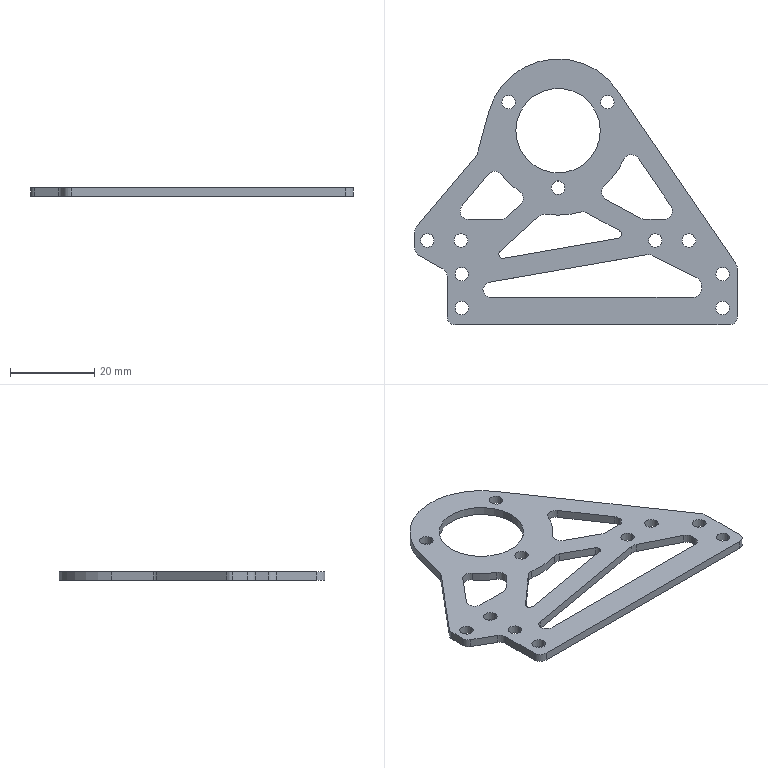Part | SolidWorks | features Fillet 4, ICE 4, Extrusion 1 | 1 solid | 78 faces | box 76.5 x 63 x 2 mm | volume 4222 mm3 | cylinder 55 | plane 23 | commonest cylinder face diameters 4 x24 3.2 x22 2 x3 34 x3 20 x2 40 x1